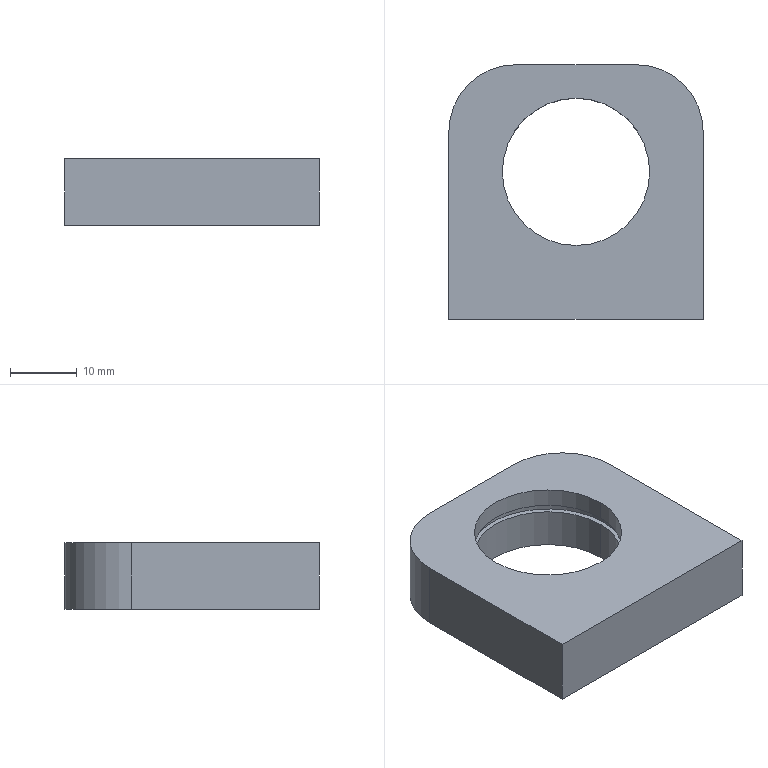Part | STEP file | 1 solid | 16 faces | box 38 x 38 x 10 mm | volume 10145 mm3 | cylinder 8 | plane 8 | commonest cylinder face diameters 22 x4 20 x2 23.5 x2
STEP:
#1=CARTESIAN_POINT('',(0.,0.,0.));
#2=DIRECTION('',(0.,0.,1.));
#3=DIRECTION('',(1.,0.,0.));
#4=AXIS2_PLACEMENT_3D('',#1,#2,#3);
#5=CARTESIAN_POINT('',(-11.75,3.,7.2));
#6=VERTEX_POINT('',#5);
#7=CARTESIAN_POINT('',(-11.75,3.,6.));
#8=VERTEX_POINT('',#7);
#9=CARTESIAN_POINT('',(-11.75,3.,7.2));
#10=DIRECTION('',(0.,0.,-1.));
#11=VECTOR('',#10,1.);
#12=LINE('',#9,#11);
#13=CARTESIAN_POINT('',(0.,3.,7.2));
#14=DIRECTION('',(0.,0.,-1.));
#15=DIRECTION('',(-1.,0.,0.));
#16=AXIS2_PLACEMENT_3D('',#13,#14,#15);
#17=CYLINDRICAL_SURFACE('',#16,11.75);
#18=CARTESIAN_POINT('',(6.283,0.));
#19=DIRECTION('',(0.,1.));
#20=VECTOR('',#19,1.);
#21=LINE('',#18,#20);
#22=(GEOMETRIC_REPRESENTATION_CONTEXT(2)PARAMETRIC_REPRESENTATION_CONTEXT()REPRESENTATION_CONTEXT('',''));
#23=DEFINITIONAL_REPRESENTATION('',(#21),#22);
#24=PCURVE('',#17,#23);
#25=CARTESIAN_POINT('',(0.,3.,7.2));
#26=DIRECTION('',(0.,0.,-1.));
#27=DIRECTION('',(-1.,0.,0.));
#28=AXIS2_PLACEMENT_3D('',#25,#26,#27);
#29=CYLINDRICAL_SURFACE('',#28,11.75);
#30=CARTESIAN_POINT('',(0.,0.));
#31=DIRECTION('',(0.,1.));
#32=VECTOR('',#31,1.);
#33=LINE('',#30,#32);
#34=(GEOMETRIC_REPRESENTATION_CONTEXT(2)PARAMETRIC_REPRESENTATION_CONTEXT()REPRESENTATION_CONTEXT('',''));
#35=DEFINITIONAL_REPRESENTATION('',(#33),#34);
#36=PCURVE('',#29,#35);
#37=SURFACE_CURVE('',#12,(#24,#36),.PCURVE_S1.);
#38=EDGE_CURVE('',#6,#8,#37,.T.);
#39=ORIENTED_EDGE('',*,*,#38,.T.);
#40=CARTESIAN_POINT('',(11.75,3.,6.));
#41=VERTEX_POINT('',#40);
#42=CARTESIAN_POINT('',(0.,3.,6.));
#43=DIRECTION('',(0.,0.,-1.));
#44=DIRECTION('',(-1.,0.,0.));
#45=AXIS2_PLACEMENT_3D('',#42,#43,#44);
#46=CIRCLE('',#45,11.75);
#47=CARTESIAN_POINT('',(0.,1.2));
#48=DIRECTION('',(1.,0.));
#49=VECTOR('',#48,1.);
#50=LINE('',#47,#49);
#51=(GEOMETRIC_REPRESENTATION_CONTEXT(2)PARAMETRIC_REPRESENTATION_CONTEXT()REPRESENTATION_CONTEXT('',''));
#52=DEFINITIONAL_REPRESENTATION('',(#50),#51);
#53=PCURVE('',#17,#52);
#54=CARTESIAN_POINT('',(0.,3.,6.));
#55=DIRECTION('',(0.,0.,-1.));
#56=DIRECTION('',(-1.,0.,0.));
#57=AXIS2_PLACEMENT_3D('',#54,#55,#56);
#58=PLANE('',#57);
#59=CARTESIAN_POINT('',(0.,0.));
#60=DIRECTION('',(1.,0.));
#61=AXIS2_PLACEMENT_2D('',#59,#60);
#62=CIRCLE('',#61,11.75);
#63=(GEOMETRIC_REPRESENTATION_CONTEXT(2)PARAMETRIC_REPRESENTATION_CONTEXT()REPRESENTATION_CONTEXT('',''));
#64=DEFINITIONAL_REPRESENTATION('',(#62),#63);
#65=PCURVE('',#58,#64);
#66=SURFACE_CURVE('',#46,(#53,#65),.PCURVE_S1.);
#67=EDGE_CURVE('',#41,#8,#66,.T.);
#68=ORIENTED_EDGE('',*,*,#67,.F.);
#69=CARTESIAN_POINT('',(11.75,3.,7.2));
#70=VERTEX_POINT('',#69);
#71=CARTESIAN_POINT('',(11.75,3.,7.2));
#72=DIRECTION('',(0.,0.,-1.));
#73=VECTOR('',#72,1.);
#74=LINE('',#71,#73);
#75=CARTESIAN_POINT('',(3.142,0.));
#76=DIRECTION('',(0.,1.));
#77=VECTOR('',#76,1.);
#78=LINE('',#75,#77);
#79=(GEOMETRIC_REPRESENTATION_CONTEXT(2)PARAMETRIC_REPRESENTATION_CONTEXT()REPRESENTATION_CONTEXT('',''));
#80=DEFINITIONAL_REPRESENTATION('',(#78),#79);
#81=PCURVE('',#17,#80);
#82=CARTESIAN_POINT('',(3.142,0.));
#83=DIRECTION('',(0.,1.));
#84=VECTOR('',#83,1.);
#85=LINE('',#82,#84);
#86=(GEOMETRIC_REPRESENTATION_CONTEXT(2)PARAMETRIC_REPRESENTATION_CONTEXT()REPRESENTATION_CONTEXT('',''));
#87=DEFINITIONAL_REPRESENTATION('',(#85),#86);
#88=PCURVE('',#29,#87);
#89=SURFACE_CURVE('',#74,(#81,#88),.PCURVE_S1.);
#90=EDGE_CURVE('',#70,#41,#89,.T.);
#91=ORIENTED_EDGE('',*,*,#90,.F.);
#92=CARTESIAN_POINT('',(0.,3.,7.2));
#93=DIRECTION('',(0.,0.,-1.));
#94=DIRECTION('',(-1.,0.,0.));
#95=AXIS2_PLACEMENT_3D('',#92,#93,#94);
#96=CIRCLE('',#95,11.75);
#97=CARTESIAN_POINT('',(0.,0.));
#98=DIRECTION('',(1.,0.));
#99=VECTOR('',#98,1.);
#100=LINE('',#97,#99);
#101=(GEOMETRIC_REPRESENTATION_CONTEXT(2)PARAMETRIC_REPRESENTATION_CONTEXT()REPRESENTATION_CONTEXT('',''));
#102=DEFINITIONAL_REPRESENTATION('',(#100),#101);
#103=PCURVE('',#17,#102);
#104=CARTESIAN_POINT('',(0.,3.,7.2));
#105=DIRECTION('',(0.,0.,-1.));
#106=DIRECTION('',(-1.,0.,0.));
#107=AXIS2_PLACEMENT_3D('',#104,#105,#106);
#108=PLANE('',#107);
#109=CARTESIAN_POINT('',(0.,0.));
#110=DIRECTION('',(1.,0.));
#111=AXIS2_PLACEMENT_2D('',#109,#110);
#112=CIRCLE('',#111,11.75);
#113=(GEOMETRIC_REPRESENTATION_CONTEXT(2)PARAMETRIC_REPRESENTATION_CONTEXT()REPRESENTATION_CONTEXT('',''));
#114=DEFINITIONAL_REPRESENTATION('',(#112),#113);
#115=PCURVE('',#108,#114);
#116=SURFACE_CURVE('',#96,(#103,#115),.PCURVE_S1.);
#117=EDGE_CURVE('',#70,#6,#116,.T.);
#118=ORIENTED_EDGE('',*,*,#117,.T.);
#119=EDGE_LOOP('',(#39,#68,#91,#118));
#120=FACE_BOUND('',#119,.F.);
#121=ADVANCED_FACE('',(#120),#17,.F.);
#122=CARTESIAN_POINT('',(-11.,3.,6.));
#123=VERTEX_POINT('',#122);
#124=CARTESIAN_POINT('',(-11.,3.,0.));
#125=VERTEX_POINT('',#124);
#126=CARTESIAN_POINT('',(-11.,3.,10.));
#127=DIRECTION('',(0.,0.,-1.));
#128=VECTOR('',#127,1.);
#129=LINE('',#126,#128);
#130=CARTESIAN_POINT('',(0.,3.,10.));
#131=DIRECTION('',(0.,0.,-1.));
#132=DIRECTION('',(-1.,0.,0.));
#133=AXIS2_PLACEMENT_3D('',#130,#131,#132);
#134=CYLINDRICAL_SURFACE('',#133,11.);
#135=CARTESIAN_POINT('',(6.283,0.));
#136=DIRECTION('',(0.,1.));
#137=VECTOR('',#136,1.);
#138=LINE('',#135,#137);
#139=(GEOMETRIC_REPRESENTATION_CONTEXT(2)PARAMETRIC_REPRESENTATION_CONTEXT()REPRESENTATION_CONTEXT('',''));
#140=DEFINITIONAL_REPRESENTATION('',(#138),#139);
#141=PCURVE('',#134,#140);
#142=CARTESIAN_POINT('',(0.,3.,10.));
#143=DIRECTION('',(0.,0.,-1.));
#144=DIRECTION('',(-1.,0.,0.));
#145=AXIS2_PLACEMENT_3D('',#142,#143,#144);
#146=CYLINDRICAL_SURFACE('',#145,11.);
#147=CARTESIAN_POINT('',(0.,0.));
#148=DIRECTION('',(0.,1.));
#149=VECTOR('',#148,1.);
#150=LINE('',#147,#149);
#151=(GEOMETRIC_REPRESENTATION_CONTEXT(2)PARAMETRIC_REPRESENTATION_CONTEXT()REPRESENTATION_CONTEXT('',''));
#152=DEFINITIONAL_REPRESENTATION('',(#150),#151);
#153=PCURVE('',#146,#152);
#154=SURFACE_CURVE('',#129,(#141,#153),.PCURVE_S1.);
#155=EDGE_CURVE('',#123,#125,#154,.T.);
#156=ORIENTED_EDGE('',*,*,#155,.T.);
#157=CARTESIAN_POINT('',(11.,3.,0.));
#158=VERTEX_POINT('',#157);
#159=CARTESIAN_POINT('',(0.,3.,0.));
#160=DIRECTION('',(0.,0.,-1.));
#161=DIRECTION('',(-1.,0.,0.));
#162=AXIS2_PLACEMENT_3D('',#159,#160,#161);
#163=CIRCLE('',#162,11.);
#164=CARTESIAN_POINT('',(0.,10.));
#165=DIRECTION('',(1.,0.));
#166=VECTOR('',#165,1.);
#167=LINE('',#164,#166);
#168=(GEOMETRIC_REPRESENTATION_CONTEXT(2)PARAMETRIC_REPRESENTATION_CONTEXT()REPRESENTATION_CONTEXT('',''));
#169=DEFINITIONAL_REPRESENTATION('',(#167),#168);
#170=PCURVE('',#134,#169);
#171=CARTESIAN_POINT('',(-9.,9.,0.));
#172=DIRECTION('',(0.,0.,1.));
#173=DIRECTION('',(1.,0.,0.));
#174=AXIS2_PLACEMENT_3D('',#171,#172,#173);
#175=PLANE('',#174);
#176=CARTESIAN_POINT('',(-2.,-6.));
#177=CARTESIAN_POINT('',(-2.,13.053));
#178=CARTESIAN_POINT('',(14.5,3.526));
#179=CARTESIAN_POINT('',(31.,-6.));
#180=CARTESIAN_POINT('',(14.5,-15.526));
#181=CARTESIAN_POINT('',(-2.,-25.053));
#182=CARTESIAN_POINT('',(-2.,-6.));
#183=(BOUNDED_CURVE()B_SPLINE_CURVE(2,(#176,#177,#178,#179,#180,#181,#182),.UNSPECIFIED.,.T.,.F.)B_SPLINE_CURVE_WITH_KNOTS((1,2,2,2,2,1),(-2.094,0.,2.094,4.189,6.283,8.378),.UNSPECIFIED.)CURVE()GEOMETRIC_REPRESENTATION_ITEM()RATIONAL_B_SPLINE_CURVE((1.,0.5,1.,0.5,1.,0.5,1.))REPRESENTATION_ITEM(''));
#184=(GEOMETRIC_REPRESENTATION_CONTEXT(2)PARAMETRIC_REPRESENTATION_CONTEXT()REPRESENTATION_CONTEXT('',''));
#185=DEFINITIONAL_REPRESENTATION('',(#183),#184);
#186=PCURVE('',#175,#185);
#187=SURFACE_CURVE('',#163,(#170,#186),.PCURVE_S1.);
#188=EDGE_CURVE('',#158,#125,#187,.T.);
#189=ORIENTED_EDGE('',*,*,#188,.F.);
#190=CARTESIAN_POINT('',(11.,3.,6.));
#191=VERTEX_POINT('',#190);
#192=CARTESIAN_POINT('',(11.,3.,10.));
#193=DIRECTION('',(0.,0.,-1.));
#194=VECTOR('',#193,1.);
#195=LINE('',#192,#194);
#196=CARTESIAN_POINT('',(3.142,0.));
#197=DIRECTION('',(0.,1.));
#198=VECTOR('',#197,1.);
#199=LINE('',#196,#198);
#200=(GEOMETRIC_REPRESENTATION_CONTEXT(2)PARAMETRIC_REPRESENTATION_CONTEXT()REPRESENTATION_CONTEXT('',''));
#201=DEFINITIONAL_REPRESENTATION('',(#199),#200);
#202=PCURVE('',#134,#201);
#203=CARTESIAN_POINT('',(3.142,0.));
#204=DIRECTION('',(0.,1.));
#205=VECTOR('',#204,1.);
#206=LINE('',#203,#205);
#207=(GEOMETRIC_REPRESENTATION_CONTEXT(2)PARAMETRIC_REPRESENTATION_CONTEXT()REPRESENTATION_CONTEXT('',''));
#208=DEFINITIONAL_REPRESENTATION('',(#206),#207);
#209=PCURVE('',#146,#208);
#210=SURFACE_CURVE('',#195,(#202,#209),.PCURVE_S1.);
#211=EDGE_CURVE('',#191,#158,#210,.T.);
#212=ORIENTED_EDGE('',*,*,#211,.F.);
#213=CARTESIAN_POINT('',(0.,3.,6.));
#214=DIRECTION('',(0.,0.,-1.));
#215=DIRECTION('',(-1.,0.,0.));
#216=AXIS2_PLACEMENT_3D('',#213,#214,#215);
#217=CIRCLE('',#216,11.);
#218=CARTESIAN_POINT('',(0.,4.));
#219=DIRECTION('',(1.,0.));
#220=VECTOR('',#219,1.);
#221=LINE('',#218,#220);
#222=(GEOMETRIC_REPRESENTATION_CONTEXT(2)PARAMETRIC_REPRESENTATION_CONTEXT()REPRESENTATION_CONTEXT('',''));
#223=DEFINITIONAL_REPRESENTATION('',(#221),#222);
#224=PCURVE('',#134,#223);
#225=CARTESIAN_POINT('',(0.,0.));
#226=DIRECTION('',(1.,0.));
#227=AXIS2_PLACEMENT_2D('',#225,#226);
#228=CIRCLE('',#227,11.);
#229=(GEOMETRIC_REPRESENTATION_CONTEXT(2)PARAMETRIC_REPRESENTATION_CONTEXT()REPRESENTATION_CONTEXT('',''));
#230=DEFINITIONAL_REPRESENTATION('',(#228),#229);
#231=PCURVE('',#58,#230);
#232=SURFACE_CURVE('',#217,(#224,#231),.PCURVE_S1.);
#233=EDGE_CURVE('',#191,#123,#232,.T.);
#234=ORIENTED_EDGE('',*,*,#233,.T.);
#235=EDGE_LOOP('',(#156,#189,#212,#234));
#236=FACE_BOUND('',#235,.F.);
#237=ADVANCED_FACE('',(#236),#134,.F.);
#238=CARTESIAN_POINT('',(-11.,3.,10.));
#239=VERTEX_POINT('',#238);
#240=CARTESIAN_POINT('',(-11.,3.,7.2));
#241=VERTEX_POINT('',#240);
#242=CARTESIAN_POINT('',(-11.,3.,10.));
#243=DIRECTION('',(0.,0.,-1.));
#244=VECTOR('',#243,1.);
#245=LINE('',#242,#244);
#246=CARTESIAN_POINT('',(0.,3.,10.));
#247=DIRECTION('',(0.,0.,-1.));
#248=DIRECTION('',(-1.,0.,0.));
#249=AXIS2_PLACEMENT_3D('',#246,#247,#248);
#250=CYLINDRICAL_SURFACE('',#249,11.);
#251=CARTESIAN_POINT('',(6.283,0.));
#252=DIRECTION('',(0.,1.));
#253=VECTOR('',#252,1.);
#254=LINE('',#251,#253);
#255=(GEOMETRIC_REPRESENTATION_CONTEXT(2)PARAMETRIC_REPRESENTATION_CONTEXT()REPRESENTATION_CONTEXT('',''));
#256=DEFINITIONAL_REPRESENTATION('',(#254),#255);
#257=PCURVE('',#250,#256);
#258=CARTESIAN_POINT('',(0.,3.,10.));
#259=DIRECTION('',(0.,0.,-1.));
#260=DIRECTION('',(-1.,0.,0.));
#261=AXIS2_PLACEMENT_3D('',#258,#259,#260);
#262=CYLINDRICAL_SURFACE('',#261,11.);
#263=CARTESIAN_POINT('',(0.,0.));
#264=DIRECTION('',(0.,1.));
#265=VECTOR('',#264,1.);
#266=LINE('',#263,#265);
#267=(GEOMETRIC_REPRESENTATION_CONTEXT(2)PARAMETRIC_REPRESENTATION_CONTEXT()REPRESENTATION_CONTEXT('',''));
#268=DEFINITIONAL_REPRESENTATION('',(#266),#267);
#269=PCURVE('',#262,#268);
#270=SURFACE_CURVE('',#245,(#257,#269),.PCURVE_S1.);
#271=EDGE_CURVE('',#239,#241,#270,.T.);
#272=ORIENTED_EDGE('',*,*,#271,.T.);
#273=CARTESIAN_POINT('',(11.,3.,7.2));
#274=VERTEX_POINT('',#273);
#275=CARTESIAN_POINT('',(0.,3.,7.2));
#276=DIRECTION('',(0.,0.,-1.));
#277=DIRECTION('',(-1.,0.,0.));
#278=AXIS2_PLACEMENT_3D('',#275,#276,#277);
#279=CIRCLE('',#278,11.);
#280=CARTESIAN_POINT('',(0.,2.8));
#281=DIRECTION('',(1.,0.));
#282=VECTOR('',#281,1.);
#283=LINE('',#280,#282);
#284=(GEOMETRIC_REPRESENTATION_CONTEXT(2)PARAMETRIC_REPRESENTATION_CONTEXT()REPRESENTATION_CONTEXT('',''));
#285=DEFINITIONAL_REPRESENTATION('',(#283),#284);
#286=PCURVE('',#250,#285);
#287=CARTESIAN_POINT('',(0.,0.));
#288=DIRECTION('',(1.,0.));
#289=AXIS2_PLACEMENT_2D('',#287,#288);
#290=CIRCLE('',#289,11.);
#291=(GEOMETRIC_REPRESENTATION_CONTEXT(2)PARAMETRIC_REPRESENTATION_CONTEXT()REPRESENTATION_CONTEXT('',''));
#292=DEFINITIONAL_REPRESENTATION('',(#290),#291);
#293=PCURVE('',#108,#292);
#294=SURFACE_CURVE('',#279,(#286,#293),.PCURVE_S1.);
#295=EDGE_CURVE('',#274,#241,#294,.T.);
#296=ORIENTED_EDGE('',*,*,#295,.F.);
#297=CARTESIAN_POINT('',(11.,3.,10.));
#298=VERTEX_POINT('',#297);
#299=CARTESIAN_POINT('',(11.,3.,10.));
#300=DIRECTION('',(0.,0.,-1.));
#301=VECTOR('',#300,1.);
#302=LINE('',#299,#301);
#303=CARTESIAN_POINT('',(3.142,0.));
#304=DIRECTION('',(0.,1.));
#305=VECTOR('',#304,1.);
#306=LINE('',#303,#305);
#307=(GEOMETRIC_REPRESENTATION_CONTEXT(2)PARAMETRIC_REPRESENTATION_CONTEXT()REPRESENTATION_CONTEXT('',''));
#308=DEFINITIONAL_REPRESENTATION('',(#306),#307);
#309=PCURVE('',#250,#308);
#310=CARTESIAN_POINT('',(3.142,0.));
#311=DIRECTION('',(0.,1.));
#312=VECTOR('',#311,1.);
#313=LINE('',#310,#312);
#314=(GEOMETRIC_REPRESENTATION_CONTEXT(2)PARAMETRIC_REPRESENTATION_CONTEXT()REPRESENTATION_CONTEXT('',''));
#315=DEFINITIONAL_REPRESENTATION('',(#313),#314);
#316=PCURVE('',#262,#315);
#317=SURFACE_CURVE('',#302,(#309,#316),.PCURVE_S1.);
#318=EDGE_CURVE('',#298,#274,#317,.T.);
#319=ORIENTED_EDGE('',*,*,#318,.F.);
#320=CARTESIAN_POINT('',(0.,3.,10.));
#321=DIRECTION('',(0.,0.,-1.));
#322=DIRECTION('',(-1.,0.,0.));
#323=AXIS2_PLACEMENT_3D('',#320,#321,#322);
#324=CIRCLE('',#323,11.);
#325=CARTESIAN_POINT('',(0.,0.));
#326=DIRECTION('',(1.,0.));
#327=VECTOR('',#326,1.);
#328=LINE('',#325,#327);
#329=(GEOMETRIC_REPRESENTATION_CONTEXT(2)PARAMETRIC_REPRESENTATION_CONTEXT()REPRESENTATION_CONTEXT('',''));
#330=DEFINITIONAL_REPRESENTATION('',(#328),#329);
#331=PCURVE('',#250,#330);
#332=CARTESIAN_POINT('',(-9.,9.,10.));
#333=DIRECTION('',(0.,0.,1.));
#334=DIRECTION('',(1.,0.,0.));
#335=AXIS2_PLACEMENT_3D('',#332,#333,#334);
#336=PLANE('',#335);
#337=CARTESIAN_POINT('',(-2.,-6.));
#338=CARTESIAN_POINT('',(-2.,13.053));
#339=CARTESIAN_POINT('',(14.5,3.526));
#340=CARTESIAN_POINT('',(31.,-6.));
#341=CARTESIAN_POINT('',(14.5,-15.526));
#342=CARTESIAN_POINT('',(-2.,-25.053));
#343=CARTESIAN_POINT('',(-2.,-6.));
#344=(BOUNDED_CURVE()B_SPLINE_CURVE(2,(#337,#338,#339,#340,#341,#342,#343),.UNSPECIFIED.,.T.,.F.)B_SPLINE_CURVE_WITH_KNOTS((1,2,2,2,2,1),(-2.094,0.,2.094,4.189,6.283,8.378),.UNSPECIFIED.)CURVE()GEOMETRIC_REPRESENTATION_ITEM()RATIONAL_B_SPLINE_CURVE((1.,0.5,1.,0.5,1.,0.5,1.))REPRESENTATION_ITEM(''));
#345=(GEOMETRIC_REPRESENTATION_CONTEXT(2)PARAMETRIC_REPRESENTATION_CONTEXT()REPRESENTATION_CONTEXT('',''));
#346=DEFINITIONAL_REPRESENTATION('',(#344),#345);
#347=PCURVE('',#336,#346);
#348=SURFACE_CURVE('',#324,(#331,#347),.PCURVE_S1.);
#349=EDGE_CURVE('',#298,#239,#348,.T.);
#350=ORIENTED_EDGE('',*,*,#349,.T.);
#351=EDGE_LOOP('',(#272,#296,#319,#350));
#352=FACE_BOUND('',#351,.F.);
#353=ADVANCED_FACE('',(#352),#250,.F.);
#354=CARTESIAN_POINT('',(0.,3.,7.2));
#355=DIRECTION('',(0.,0.,-1.));
#356=DIRECTION('',(-1.,0.,0.));
#357=AXIS2_PLACEMENT_3D('',#354,#355,#356);
#358=CIRCLE('',#357,11.);
#359=CARTESIAN_POINT('',(0.,2.8));
#360=DIRECTION('',(1.,0.));
#361=VECTOR('',#360,1.);
#362=LINE('',#359,#361);
#363=(GEOMETRIC_REPRESENTATION_CONTEXT(2)PARAMETRIC_REPRESENTATION_CONTEXT()REPRESENTATION_CONTEXT('',''));
#364=DEFINITIONAL_REPRESENTATION('',(#362),#363);
#365=PCURVE('',#262,#364);
#366=CARTESIAN_POINT('',(0.,0.));
#367=DIRECTION('',(1.,0.));
#368=AXIS2_PLACEMENT_2D('',#366,#367);
#369=CIRCLE('',#368,11.);
#370=(GEOMETRIC_REPRESENTATION_CONTEXT(2)PARAMETRIC_REPRESENTATION_CONTEXT()REPRESENTATION_CONTEXT('',''));
#371=DEFINITIONAL_REPRESENTATION('',(#369),#370);
#372=PCURVE('',#108,#371);
#373=SURFACE_CURVE('',#358,(#365,#372),.PCURVE_S1.);
#374=EDGE_CURVE('',#241,#274,#373,.T.);
#375=ORIENTED_EDGE('',*,*,#374,.F.);
#376=ORIENTED_EDGE('',*,*,#271,.F.);
#377=CARTESIAN_POINT('',(0.,3.,10.));
#378=DIRECTION('',(0.,0.,-1.));
#379=DIRECTION('',(-1.,0.,0.));
#380=AXIS2_PLACEMENT_3D('',#377,#378,#379);
#381=CIRCLE('',#380,11.);
#382=CARTESIAN_POINT('',(0.,0.));
#383=DIRECTION('',(1.,0.));
#384=VECTOR('',#383,1.);
#385=LINE('',#382,#384);
#386=(GEOMETRIC_REPRESENTATION_CONTEXT(2)PARAMETRIC_REPRESENTATION_CONTEXT()REPRESENTATION_CONTEXT('',''));
#387=DEFINITIONAL_REPRESENTATION('',(#385),#386);
#388=PCURVE('',#262,#387);
#389=CARTESIAN_POINT('',(-2.,-6.));
#390=CARTESIAN_POINT('',(-2.,13.053));
#391=CARTESIAN_POINT('',(14.5,3.526));
#392=CARTESIAN_POINT('',(31.,-6.));
#393=CARTESIAN_POINT('',(14.5,-15.526));
#394=CARTESIAN_POINT('',(-2.,-25.053));
#395=CARTESIAN_POINT('',(-2.,-6.));
#396=(BOUNDED_CURVE()B_SPLINE_CURVE(2,(#389,#390,#391,#392,#393,#394,#395),.UNSPECIFIED.,.T.,.F.)B_SPLINE_CURVE_WITH_KNOTS((1,2,2,2,2,1),(-2.094,0.,2.094,4.189,6.283,8.378),.UNSPECIFIED.)CURVE()GEOMETRIC_REPRESENTATION_ITEM()RATIONAL_B_SPLINE_CURVE((1.,0.5,1.,0.5,1.,0.5,1.))REPRESENTATION_ITEM(''));
#397=(GEOMETRIC_REPRESENTATION_CONTEXT(2)PARAMETRIC_REPRESENTATION_CONTEXT()REPRESENTATION_CONTEXT('',''));
#398=DEFINITIONAL_REPRESENTATION('',(#396),#397);
#399=PCURVE('',#336,#398);
#400=SURFACE_CURVE('',#381,(#388,#399),.PCURVE_S1.);
#401=EDGE_CURVE('',#239,#298,#400,.T.);
#402=ORIENTED_EDGE('',*,*,#401,.T.);
#403=ORIENTED_EDGE('',*,*,#318,.T.);
#404=EDGE_LOOP('',(#375,#376,#402,#403));
#405=FACE_BOUND('',#404,.F.);
#406=ADVANCED_FACE('',(#405),#262,.F.);
#407=CARTESIAN_POINT('',(19.,-19.,0.));
#408=VERTEX_POINT('',#407);
#409=CARTESIAN_POINT('',(19.,9.,0.));
#410=VERTEX_POINT('',#409);
#411=CARTESIAN_POINT('',(19.,9.,0.));
#412=DIRECTION('',(0.,1.,0.));
#413=VECTOR('',#412,1.);
#414=LINE('',#411,#413);
#415=CARTESIAN_POINT('',(19.,9.,10.));
#416=DIRECTION('',(-1.,0.,0.));
#417=DIRECTION('',(0.,-1.,0.));
#418=AXIS2_PLACEMENT_3D('',#415,#416,#417);
#419=PLANE('',#418);
#420=CARTESIAN_POINT('',(0.,-10.));
#421=DIRECTION('',(-1.,0.));
#422=VECTOR('',#421,1.);
#423=LINE('',#420,#422);
#424=(GEOMETRIC_REPRESENTATION_CONTEXT(2)PARAMETRIC_REPRESENTATION_CONTEXT()REPRESENTATION_CONTEXT('',''));
#425=DEFINITIONAL_REPRESENTATION('',(#423),#424);
#426=PCURVE('',#419,#425);
#427=CARTESIAN_POINT('',(28.,0.));
#428=DIRECTION('',(0.,1.));
#429=VECTOR('',#428,1.);
#430=LINE('',#427,#429);
#431=(GEOMETRIC_REPRESENTATION_CONTEXT(2)PARAMETRIC_REPRESENTATION_CONTEXT()REPRESENTATION_CONTEXT('',''));
#432=DEFINITIONAL_REPRESENTATION('',(#430),#431);
#433=PCURVE('',#175,#432);
#434=SURFACE_CURVE('',#414,(#426,#433),.PCURVE_S1.);
#435=EDGE_CURVE('',#408,#410,#434,.T.);
#436=ORIENTED_EDGE('',*,*,#435,.T.);
#437=CARTESIAN_POINT('',(19.,9.,10.));
#438=VERTEX_POINT('',#437);
#439=CARTESIAN_POINT('',(19.,9.,10.));
#440=DIRECTION('',(0.,0.,-1.));
#441=VECTOR('',#440,1.);
#442=LINE('',#439,#441);
#443=CARTESIAN_POINT('',(0.,0.));
#444=DIRECTION('',(0.,-1.));
#445=VECTOR('',#444,1.);
#446=LINE('',#443,#445);
#447=(GEOMETRIC_REPRESENTATION_CONTEXT(2)PARAMETRIC_REPRESENTATION_CONTEXT()REPRESENTATION_CONTEXT('',''));
#448=DEFINITIONAL_REPRESENTATION('',(#446),#447);
#449=PCURVE('',#419,#448);
#450=CARTESIAN_POINT('',(9.,9.,10.));
#451=DIRECTION('',(0.,0.,-1.));
#452=DIRECTION('',(-1.,0.,0.));
#453=AXIS2_PLACEMENT_3D('',#450,#451,#452);
#454=CYLINDRICAL_SURFACE('',#453,10.);
#455=CARTESIAN_POINT('',(3.142,0.));
#456=DIRECTION('',(0.,1.));
#457=VECTOR('',#456,1.);
#458=LINE('',#455,#457);
#459=(GEOMETRIC_REPRESENTATION_CONTEXT(2)PARAMETRIC_REPRESENTATION_CONTEXT()REPRESENTATION_CONTEXT('',''));
#460=DEFINITIONAL_REPRESENTATION('',(#458),#459);
#461=PCURVE('',#454,#460);
#462=SURFACE_CURVE('',#442,(#449,#461),.PCURVE_S1.);
#463=EDGE_CURVE('',#438,#410,#462,.T.);
#464=ORIENTED_EDGE('',*,*,#463,.F.);
#465=CARTESIAN_POINT('',(19.,-19.,10.));
#466=VERTEX_POINT('',#465);
#467=CARTESIAN_POINT('',(19.,9.,10.));
#468=DIRECTION('',(0.,1.,0.));
#469=VECTOR('',#468,1.);
#470=LINE('',#467,#469);
#471=CARTESIAN_POINT('',(0.,0.));
#472=DIRECTION('',(-1.,0.));
#473=VECTOR('',#472,1.);
#474=LINE('',#471,#473);
#475=(GEOMETRIC_REPRESENTATION_CONTEXT(2)PARAMETRIC_REPRESENTATION_CONTEXT()REPRESENTATION_CONTEXT('',''));
#476=DEFINITIONAL_REPRESENTATION('',(#474),#475);
#477=PCURVE('',#419,#476);
#478=CARTESIAN_POINT('',(28.,0.));
#479=DIRECTION('',(0.,1.));
#480=VECTOR('',#479,1.);
#481=LINE('',#478,#480);
#482=(GEOMETRIC_REPRESENTATION_CONTEXT(2)PARAMETRIC_REPRESENTATION_CONTEXT()REPRESENTATION_CONTEXT('',''));
#483=DEFINITIONAL_REPRESENTATION('',(#481),#482);
#484=PCURVE('',#336,#483);
#485=SURFACE_CURVE('',#470,(#477,#484),.PCURVE_S1.);
#486=EDGE_CURVE('',#466,#438,#485,.T.);
#487=ORIENTED_EDGE('',*,*,#486,.F.);
#488=CARTESIAN_POINT('',(19.,-19.,10.));
#489=DIRECTION('',(0.,0.,-1.));
#490=VECTOR('',#489,1.);
#491=LINE('',#488,#490);
#492=CARTESIAN_POINT('',(28.,0.));
#493=DIRECTION('',(0.,-1.));
#494=VECTOR('',#493,1.);
#495=LINE('',#492,#494);
#496=(GEOMETRIC_REPRESENTATION_CONTEXT(2)PARAMETRIC_REPRESENTATION_CONTEXT()REPRESENTATION_CONTEXT('',''));
#497=DEFINITIONAL_REPRESENTATION('',(#495),#496);
#498=PCURVE('',#419,#497);
#499=CARTESIAN_POINT('',(-19.,-19.,10.));
#500=DIRECTION('',(0.,1.,0.));
#501=DIRECTION('',(0.,0.,1.));
#502=AXIS2_PLACEMENT_3D('',#499,#500,#501);
#503=PLANE('',#502);
#504=CARTESIAN_POINT('',(0.,38.));
#505=DIRECTION('',(-1.,0.));
#506=VECTOR('',#505,1.);
#507=LINE('',#504,#506);
#508=(GEOMETRIC_REPRESENTATION_CONTEXT(2)PARAMETRIC_REPRESENTATION_CONTEXT()REPRESENTATION_CONTEXT('',''));
#509=DEFINITIONAL_REPRESENTATION('',(#507),#508);
#510=PCURVE('',#503,#509);
#511=SURFACE_CURVE('',#491,(#498,#510),.PCURVE_S1.);
#512=EDGE_CURVE('',#466,#408,#511,.T.);
#513=ORIENTED_EDGE('',*,*,#512,.T.);
#514=EDGE_LOOP('',(#436,#464,#487,#513));
#515=FACE_BOUND('',#514,.T.);
#516=ADVANCED_FACE('',(#515),#419,.F.);
#517=CARTESIAN_POINT('',(9.,19.,0.));
#518=VERTEX_POINT('',#517);
#519=CARTESIAN_POINT('',(9.,9.,0.));
#520=DIRECTION('',(0.,0.,1.));
#521=DIRECTION('',(-1.,0.,0.));
#522=AXIS2_PLACEMENT_3D('',#519,#520,#521);
#523=CIRCLE('',#522,10.);
#524=CARTESIAN_POINT('',(6.283,10.));
#525=DIRECTION('',(-1.,0.));
#526=VECTOR('',#525,1.);
#527=LINE('',#524,#526);
#528=(GEOMETRIC_REPRESENTATION_CONTEXT(2)PARAMETRIC_REPRESENTATION_CONTEXT()REPRESENTATION_CONTEXT('',''));
#529=DEFINITIONAL_REPRESENTATION('',(#527),#528);
#530=PCURVE('',#454,#529);
#531=CARTESIAN_POINT('',(18.,0.));
#532=DIRECTION('',(-1.,0.));
#533=AXIS2_PLACEMENT_2D('',#531,#532);
#534=CIRCLE('',#533,10.);
#535=(GEOMETRIC_REPRESENTATION_CONTEXT(2)PARAMETRIC_REPRESENTATION_CONTEXT()REPRESENTATION_CONTEXT('',''));
#536=DEFINITIONAL_REPRESENTATION('',(#534),#535);
#537=PCURVE('',#175,#536);
#538=SURFACE_CURVE('',#523,(#530,#537),.PCURVE_S1.);
#539=EDGE_CURVE('',#410,#518,#538,.T.);
#540=ORIENTED_EDGE('',*,*,#539,.T.);
#541=CARTESIAN_POINT('',(9.,19.,10.));
#542=VERTEX_POINT('',#541);
#543=CARTESIAN_POINT('',(9.,19.,10.));
#544=DIRECTION('',(0.,0.,-1.));
#545=VECTOR('',#544,1.);
#546=LINE('',#543,#545);
#547=CARTESIAN_POINT('',(1.571,0.));
#548=DIRECTION('',(0.,1.));
#549=VECTOR('',#548,1.);
#550=LINE('',#547,#549);
#551=(GEOMETRIC_REPRESENTATION_CONTEXT(2)PARAMETRIC_REPRESENTATION_CONTEXT()REPRESENTATION_CONTEXT('',''));
#552=DEFINITIONAL_REPRESENTATION('',(#550),#551);
#553=PCURVE('',#454,#552);
#554=CARTESIAN_POINT('',(-9.,19.,10.));
#555=DIRECTION('',(0.,-1.,0.));
#556=DIRECTION('',(1.,0.,0.));
#557=AXIS2_PLACEMENT_3D('',#554,#555,#556);
#558=PLANE('',#557);
#559=CARTESIAN_POINT('',(18.,0.));
#560=DIRECTION('',(0.,-1.));
#561=VECTOR('',#560,1.);
#562=LINE('',#559,#561);
#563=(GEOMETRIC_REPRESENTATION_CONTEXT(2)PARAMETRIC_REPRESENTATION_CONTEXT()REPRESENTATION_CONTEXT('',''));
#564=DEFINITIONAL_REPRESENTATION('',(#562),#563);
#565=PCURVE('',#558,#564);
#566=SURFACE_CURVE('',#546,(#553,#565),.PCURVE_S1.);
#567=EDGE_CURVE('',#542,#518,#566,.T.);
#568=ORIENTED_EDGE('',*,*,#567,.F.);
#569=CARTESIAN_POINT('',(9.,9.,10.));
#570=DIRECTION('',(0.,0.,1.));
#571=DIRECTION('',(-1.,0.,0.));
#572=AXIS2_PLACEMENT_3D('',#569,#570,#571);
#573=CIRCLE('',#572,10.);
#574=CARTESIAN_POINT('',(6.283,0.));
#575=DIRECTION('',(-1.,0.));
#576=VECTOR('',#575,1.);
#577=LINE('',#574,#576);
#578=(GEOMETRIC_REPRESENTATION_CONTEXT(2)PARAMETRIC_REPRESENTATION_CONTEXT()REPRESENTATION_CONTEXT('',''));
#579=DEFINITIONAL_REPRESENTATION('',(#577),#578);
#580=PCURVE('',#454,#579);
#581=CARTESIAN_POINT('',(18.,0.));
#582=DIRECTION('',(-1.,0.));
#583=AXIS2_PLACEMENT_2D('',#581,#582);
#584=CIRCLE('',#583,10.);
#585=(GEOMETRIC_REPRESENTATION_CONTEXT(2)PARAMETRIC_REPRESENTATION_CONTEXT()REPRESENTATION_CONTEXT('',''));
#586=DEFINITIONAL_REPRESENTATION('',(#584),#585);
#587=PCURVE('',#336,#586);
#588=SURFACE_CURVE('',#573,(#580,#587),.PCURVE_S1.);
#589=EDGE_CURVE('',#438,#542,#588,.T.);
#590=ORIENTED_EDGE('',*,*,#589,.F.);
#591=ORIENTED_EDGE('',*,*,#463,.T.);
#592=EDGE_LOOP('',(#540,#568,#590,#591));
#593=FACE_BOUND('',#592,.T.);
#594=ADVANCED_FACE('',(#593),#454,.T.);
#595=CARTESIAN_POINT('',(-9.,19.,0.));
#596=VERTEX_POINT('',#595);
#597=CARTESIAN_POINT('',(-9.,19.,0.));
#598=DIRECTION('',(-1.,0.,0.));
#599=VECTOR('',#598,1.);
#600=LINE('',#597,#599);
#601=CARTESIAN_POINT('',(0.,-10.));
#602=DIRECTION('',(-1.,0.));
#603=VECTOR('',#602,1.);
#604=LINE('',#601,#603);
#605=(GEOMETRIC_REPRESENTATION_CONTEXT(2)PARAMETRIC_REPRESENTATION_CONTEXT()REPRESENTATION_CONTEXT('',''));
#606=DEFINITIONAL_REPRESENTATION('',(#604),#605);
#607=PCURVE('',#558,#606);
#608=CARTESIAN_POINT('',(0.,10.));
#609=DIRECTION('',(-1.,0.));
#610=VECTOR('',#609,1.);
#611=LINE('',#608,#610);
#612=(GEOMETRIC_REPRESENTATION_CONTEXT(2)PARAMETRIC_REPRESENTATION_CONTEXT()REPRESENTATION_CONTEXT('',''));
#613=DEFINITIONAL_REPRESENTATION('',(#611),#612);
#614=PCURVE('',#175,#613);
#615=SURFACE_CURVE('',#600,(#607,#614),.PCURVE_S1.);
#616=EDGE_CURVE('',#518,#596,#615,.T.);
#617=ORIENTED_EDGE('',*,*,#616,.T.);
#618=CARTESIAN_POINT('',(-9.,19.,10.));
#619=VERTEX_POINT('',#618);
#620=CARTESIAN_POINT('',(-9.,19.,10.));
#621=DIRECTION('',(0.,0.,-1.));
#622=VECTOR('',#621,1.);
#623=LINE('',#620,#622);
#624=CARTESIAN_POINT('',(0.,0.));
#625=DIRECTION('',(0.,-1.));
#626=VECTOR('',#625,1.);
#627=LINE('',#624,#626);
#628=(GEOMETRIC_REPRESENTATION_CONTEXT(2)PARAMETRIC_REPRESENTATION_CONTEXT()REPRESENTATION_CONTEXT('',''));
#629=DEFINITIONAL_REPRESENTATION('',(#627),#628);
#630=PCURVE('',#558,#629);
#631=CARTESIAN_POINT('',(-9.,9.,10.));
#632=DIRECTION('',(0.,0.,-1.));
#633=DIRECTION('',(-1.,0.,0.));
#634=AXIS2_PLACEMENT_3D('',#631,#632,#633);
#635=CYLINDRICAL_SURFACE('',#634,10.);
#636=CARTESIAN_POINT('',(1.571,0.));
#637=DIRECTION('',(0.,1.));
#638=VECTOR('',#637,1.);
#639=LINE('',#636,#638);
#640=(GEOMETRIC_REPRESENTATION_CONTEXT(2)PARAMETRIC_REPRESENTATION_CONTEXT()REPRESENTATION_CONTEXT('',''));
#641=DEFINITIONAL_REPRESENTATION('',(#639),#640);
#642=PCURVE('',#635,#641);
#643=SURFACE_CURVE('',#623,(#630,#642),.PCURVE_S1.);
#644=EDGE_CURVE('',#619,#596,#643,.T.);
#645=ORIENTED_EDGE('',*,*,#644,.F.);
#646=CARTESIAN_POINT('',(-9.,19.,10.));
#647=DIRECTION('',(-1.,0.,0.));
#648=VECTOR('',#647,1.);
#649=LINE('',#646,#648);
#650=CARTESIAN_POINT('',(0.,0.));
#651=DIRECTION('',(-1.,0.));
#652=VECTOR('',#651,1.);
#653=LINE('',#650,#652);
#654=(GEOMETRIC_REPRESENTATION_CONTEXT(2)PARAMETRIC_REPRESENTATION_CONTEXT()REPRESENTATION_CONTEXT('',''));
#655=DEFINITIONAL_REPRESENTATION('',(#653),#654);
#656=PCURVE('',#558,#655);
#657=CARTESIAN_POINT('',(0.,10.));
#658=DIRECTION('',(-1.,0.));
#659=VECTOR('',#658,1.);
#660=LINE('',#657,#659);
#661=(GEOMETRIC_REPRESENTATION_CONTEXT(2)PARAMETRIC_REPRESENTATION_CONTEXT()REPRESENTATION_CONTEXT('',''));
#662=DEFINITIONAL_REPRESENTATION('',(#660),#661);
#663=PCURVE('',#336,#662);
#664=SURFACE_CURVE('',#649,(#656,#663),.PCURVE_S1.);
#665=EDGE_CURVE('',#542,#619,#664,.T.);
#666=ORIENTED_EDGE('',*,*,#665,.F.);
#667=ORIENTED_EDGE('',*,*,#567,.T.);
#668=EDGE_LOOP('',(#617,#645,#666,#667));
#669=FACE_BOUND('',#668,.T.);
#670=ADVANCED_FACE('',(#669),#558,.F.);
#671=CARTESIAN_POINT('',(-19.,9.,0.));
#672=VERTEX_POINT('',#671);
#673=CARTESIAN_POINT('',(-9.,9.,0.));
#674=DIRECTION('',(0.,0.,1.));
#675=DIRECTION('',(1.,0.,0.));
#676=AXIS2_PLACEMENT_3D('',#673,#674,#675);
#677=CIRCLE('',#676,10.);
#678=CARTESIAN_POINT('',(3.142,10.));
#679=DIRECTION('',(-1.,0.));
#680=VECTOR('',#679,1.);
#681=LINE('',#678,#680);
#682=(GEOMETRIC_REPRESENTATION_CONTEXT(2)PARAMETRIC_REPRESENTATION_CONTEXT()REPRESENTATION_CONTEXT('',''));
#683=DEFINITIONAL_REPRESENTATION('',(#681),#682);
#684=PCURVE('',#635,#683);
#685=CARTESIAN_POINT('',(0.,0.));
#686=DIRECTION('',(1.,0.));
#687=AXIS2_PLACEMENT_2D('',#685,#686);
#688=CIRCLE('',#687,10.);
#689=(GEOMETRIC_REPRESENTATION_CONTEXT(2)PARAMETRIC_REPRESENTATION_CONTEXT()REPRESENTATION_CONTEXT('',''));
#690=DEFINITIONAL_REPRESENTATION('',(#688),#689);
#691=PCURVE('',#175,#690);
#692=SURFACE_CURVE('',#677,(#684,#691),.PCURVE_S1.);
#693=EDGE_CURVE('',#596,#672,#692,.T.);
#694=ORIENTED_EDGE('',*,*,#693,.T.);
#695=CARTESIAN_POINT('',(-19.,9.,10.));
#696=VERTEX_POINT('',#695);
#697=CARTESIAN_POINT('',(-19.,9.,10.));
#698=DIRECTION('',(0.,0.,-1.));
#699=VECTOR('',#698,1.);
#700=LINE('',#697,#699);
#701=CARTESIAN_POINT('',(0.,0.));
#702=DIRECTION('',(0.,1.));
#703=VECTOR('',#702,1.);
#704=LINE('',#701,#703);
#705=(GEOMETRIC_REPRESENTATION_CONTEXT(2)PARAMETRIC_REPRESENTATION_CONTEXT()REPRESENTATION_CONTEXT('',''));
#706=DEFINITIONAL_REPRESENTATION('',(#704),#705);
#707=PCURVE('',#635,#706);
#708=CARTESIAN_POINT('',(-19.,9.,10.));
#709=DIRECTION('',(1.,0.,0.));
#710=DIRECTION('',(0.,1.,0.));
#711=AXIS2_PLACEMENT_3D('',#708,#709,#710);
#712=PLANE('',#711);
#713=CARTESIAN_POINT('',(0.,0.));
#714=DIRECTION('',(0.,-1.));
#715=VECTOR('',#714,1.);
#716=LINE('',#713,#715);
#717=(GEOMETRIC_REPRESENTATION_CONTEXT(2)PARAMETRIC_REPRESENTATION_CONTEXT()REPRESENTATION_CONTEXT('',''));
#718=DEFINITIONAL_REPRESENTATION('',(#716),#717);
#719=PCURVE('',#712,#718);
#720=SURFACE_CURVE('',#700,(#707,#719),.PCURVE_S1.);
#721=EDGE_CURVE('',#696,#672,#720,.T.);
#722=ORIENTED_EDGE('',*,*,#721,.F.);
#723=CARTESIAN_POINT('',(-9.,9.,10.));
#724=DIRECTION('',(0.,0.,1.));
#725=DIRECTION('',(1.,0.,0.));
#726=AXIS2_PLACEMENT_3D('',#723,#724,#725);
#727=CIRCLE('',#726,10.);
#728=CARTESIAN_POINT('',(3.142,0.));
#729=DIRECTION('',(-1.,0.));
#730=VECTOR('',#729,1.);
#731=LINE('',#728,#730);
#732=(GEOMETRIC_REPRESENTATION_CONTEXT(2)PARAMETRIC_REPRESENTATION_CONTEXT()REPRESENTATION_CONTEXT('',''));
#733=DEFINITIONAL_REPRESENTATION('',(#731),#732);
#734=PCURVE('',#635,#733);
#735=CARTESIAN_POINT('',(0.,0.));
#736=DIRECTION('',(1.,0.));
#737=AXIS2_PLACEMENT_2D('',#735,#736);
#738=CIRCLE('',#737,10.);
#739=(GEOMETRIC_REPRESENTATION_CONTEXT(2)PARAMETRIC_REPRESENTATION_CONTEXT()REPRESENTATION_CONTEXT('',''));
#740=DEFINITIONAL_REPRESENTATION('',(#738),#739);
#741=PCURVE('',#336,#740);
#742=SURFACE_CURVE('',#727,(#734,#741),.PCURVE_S1.);
#743=EDGE_CURVE('',#619,#696,#742,.T.);
#744=ORIENTED_EDGE('',*,*,#743,.F.);
#745=ORIENTED_EDGE('',*,*,#644,.T.);
#746=EDGE_LOOP('',(#694,#722,#744,#745));
#747=FACE_BOUND('',#746,.T.);
#748=ADVANCED_FACE('',(#747),#635,.T.);
#749=CARTESIAN_POINT('',(-19.,-19.,0.));
#750=VERTEX_POINT('',#749);
#751=CARTESIAN_POINT('',(-19.,9.,0.));
#752=DIRECTION('',(0.,-1.,0.));
#753=VECTOR('',#752,1.);
#754=LINE('',#751,#753);
#755=CARTESIAN_POINT('',(0.,-10.));
#756=DIRECTION('',(-1.,0.));
#757=VECTOR('',#756,1.);
#758=LINE('',#755,#757);
#759=(GEOMETRIC_REPRESENTATION_CONTEXT(2)PARAMETRIC_REPRESENTATION_CONTEXT()REPRESENTATION_CONTEXT('',''));
#760=DEFINITIONAL_REPRESENTATION('',(#758),#759);
#761=PCURVE('',#712,#760);
#762=CARTESIAN_POINT('',(-10.,0.));
#763=DIRECTION('',(0.,-1.));
#764=VECTOR('',#763,1.);
#765=LINE('',#762,#764);
#766=(GEOMETRIC_REPRESENTATION_CONTEXT(2)PARAMETRIC_REPRESENTATION_CONTEXT()REPRESENTATION_CONTEXT('',''));
#767=DEFINITIONAL_REPRESENTATION('',(#765),#766);
#768=PCURVE('',#175,#767);
#769=SURFACE_CURVE('',#754,(#761,#768),.PCURVE_S1.);
#770=EDGE_CURVE('',#672,#750,#769,.T.);
#771=ORIENTED_EDGE('',*,*,#770,.T.);
#772=CARTESIAN_POINT('',(-19.,-19.,10.));
#773=VERTEX_POINT('',#772);
#774=CARTESIAN_POINT('',(-19.,-19.,10.));
#775=DIRECTION('',(0.,0.,-1.));
#776=VECTOR('',#775,1.);
#777=LINE('',#774,#776);
#778=CARTESIAN_POINT('',(-28.,0.));
#779=DIRECTION('',(0.,-1.));
#780=VECTOR('',#779,1.);
#781=LINE('',#778,#780);
#782=(GEOMETRIC_REPRESENTATION_CONTEXT(2)PARAMETRIC_REPRESENTATION_CONTEXT()REPRESENTATION_CONTEXT('',''));
#783=DEFINITIONAL_REPRESENTATION('',(#781),#782);
#784=PCURVE('',#712,#783);
#785=CARTESIAN_POINT('',(0.,0.));
#786=DIRECTION('',(-1.,0.));
#787=VECTOR('',#786,1.);
#788=LINE('',#785,#787);
#789=(GEOMETRIC_REPRESENTATION_CONTEXT(2)PARAMETRIC_REPRESENTATION_CONTEXT()REPRESENTATION_CONTEXT('',''));
#790=DEFINITIONAL_REPRESENTATION('',(#788),#789);
#791=PCURVE('',#503,#790);
#792=SURFACE_CURVE('',#777,(#784,#791),.PCURVE_S1.);
#793=EDGE_CURVE('',#773,#750,#792,.T.);
#794=ORIENTED_EDGE('',*,*,#793,.F.);
#795=CARTESIAN_POINT('',(-19.,9.,10.));
#796=DIRECTION('',(0.,-1.,0.));
#797=VECTOR('',#796,1.);
#798=LINE('',#795,#797);
#799=CARTESIAN_POINT('',(0.,0.));
#800=DIRECTION('',(-1.,0.));
#801=VECTOR('',#800,1.);
#802=LINE('',#799,#801);
#803=(GEOMETRIC_REPRESENTATION_CONTEXT(2)PARAMETRIC_REPRESENTATION_CONTEXT()REPRESENTATION_CONTEXT('',''));
#804=DEFINITIONAL_REPRESENTATION('',(#802),#803);
#805=PCURVE('',#712,#804);
#806=CARTESIAN_POINT('',(-10.,0.));
#807=DIRECTION('',(0.,-1.));
#808=VECTOR('',#807,1.);
#809=LINE('',#806,#808);
#810=(GEOMETRIC_REPRESENTATION_CONTEXT(2)PARAMETRIC_REPRESENTATION_CONTEXT()REPRESENTATION_CONTEXT('',''));
#811=DEFINITIONAL_REPRESENTATION('',(#809),#810);
#812=PCURVE('',#336,#811);
#813=SURFACE_CURVE('',#798,(#805,#812),.PCURVE_S1.);
#814=EDGE_CURVE('',#696,#773,#813,.T.);
#815=ORIENTED_EDGE('',*,*,#814,.F.);
#816=ORIENTED_EDGE('',*,*,#721,.T.);
#817=EDGE_LOOP('',(#771,#794,#815,#816));
#818=FACE_BOUND('',#817,.T.);
#819=ADVANCED_FACE('',(#818),#712,.F.);
#820=CARTESIAN_POINT('',(-19.,-19.,0.));
#821=DIRECTION('',(1.,0.,0.));
#822=VECTOR('',#821,1.);
#823=LINE('',#820,#822);
#824=CARTESIAN_POINT('',(-10.,0.));
#825=DIRECTION('',(0.,1.));
#826=VECTOR('',#825,1.);
#827=LINE('',#824,#826);
#828=(GEOMETRIC_REPRESENTATION_CONTEXT(2)PARAMETRIC_REPRESENTATION_CONTEXT()REPRESENTATION_CONTEXT('',''));
#829=DEFINITIONAL_REPRESENTATION('',(#827),#828);
#830=PCURVE('',#503,#829);
#831=CARTESIAN_POINT('',(-10.,-28.));
#832=DIRECTION('',(1.,0.));
#833=VECTOR('',#832,1.);
#834=LINE('',#831,#833);
#835=(GEOMETRIC_REPRESENTATION_CONTEXT(2)PARAMETRIC_REPRESENTATION_CONTEXT()REPRESENTATION_CONTEXT('',''));
#836=DEFINITIONAL_REPRESENTATION('',(#834),#835);
#837=PCURVE('',#175,#836);
#838=SURFACE_CURVE('',#823,(#830,#837),.PCURVE_S1.);
#839=EDGE_CURVE('',#750,#408,#838,.T.);
#840=ORIENTED_EDGE('',*,*,#839,.T.);
#841=ORIENTED_EDGE('',*,*,#512,.F.);
#842=CARTESIAN_POINT('',(-19.,-19.,10.));
#843=DIRECTION('',(1.,0.,0.));
#844=VECTOR('',#843,1.);
#845=LINE('',#842,#844);
#846=CARTESIAN_POINT('',(0.,0.));
#847=DIRECTION('',(0.,1.));
#848=VECTOR('',#847,1.);
#849=LINE('',#846,#848);
#850=(GEOMETRIC_REPRESENTATION_CONTEXT(2)PARAMETRIC_REPRESENTATION_CONTEXT()REPRESENTATION_CONTEXT('',''));
#851=DEFINITIONAL_REPRESENTATION('',(#849),#850);
#852=PCURVE('',#503,#851);
#853=CARTESIAN_POINT('',(-10.,-28.));
#854=DIRECTION('',(1.,0.));
#855=VECTOR('',#854,1.);
#856=LINE('',#853,#855);
#857=(GEOMETRIC_REPRESENTATION_CONTEXT(2)PARAMETRIC_REPRESENTATION_CONTEXT()REPRESENTATION_CONTEXT('',''));
#858=DEFINITIONAL_REPRESENTATION('',(#856),#857);
#859=PCURVE('',#336,#858);
#860=SURFACE_CURVE('',#845,(#852,#859),.PCURVE_S1.);
#861=EDGE_CURVE('',#773,#466,#860,.T.);
#862=ORIENTED_EDGE('',*,*,#861,.F.);
#863=ORIENTED_EDGE('',*,*,#793,.T.);
#864=EDGE_LOOP('',(#840,#841,#862,#863));
#865=FACE_BOUND('',#864,.T.);
#866=ADVANCED_FACE('',(#865),#503,.F.);
#867=ORIENTED_EDGE('',*,*,#401,.T.);
#868=ORIENTED_EDGE('',*,*,#349,.T.);
#869=EDGE_LOOP('',(#867,#868));
#870=FACE_BOUND('',#869,.T.);
#871=ORIENTED_EDGE('',*,*,#486,.T.);
#872=ORIENTED_EDGE('',*,*,#589,.T.);
#873=ORIENTED_EDGE('',*,*,#665,.T.);
#874=ORIENTED_EDGE('',*,*,#743,.T.);
#875=ORIENTED_EDGE('',*,*,#814,.T.);
#876=ORIENTED_EDGE('',*,*,#861,.T.);
#877=EDGE_LOOP('',(#871,#872,#873,#874,#875,#876));
#878=FACE_BOUND('',#877,.T.);
#879=ADVANCED_FACE('',(#870,#878),#336,.T.);
#880=CARTESIAN_POINT('',(0.,3.,0.));
#881=DIRECTION('',(0.,0.,-1.));
#882=DIRECTION('',(-1.,0.,0.));
#883=AXIS2_PLACEMENT_3D('',#880,#881,#882);
#884=CIRCLE('',#883,11.);
#885=CARTESIAN_POINT('',(-2.,-6.));
#886=CARTESIAN_POINT('',(-2.,13.053));
#887=CARTESIAN_POINT('',(14.5,3.526));
#888=CARTESIAN_POINT('',(31.,-6.));
#889=CARTESIAN_POINT('',(14.5,-15.526));
#890=CARTESIAN_POINT('',(-2.,-25.053));
#891=CARTESIAN_POINT('',(-2.,-6.));
#892=(BOUNDED_CURVE()B_SPLINE_CURVE(2,(#885,#886,#887,#888,#889,#890,#891),.UNSPECIFIED.,.T.,.F.)B_SPLINE_CURVE_WITH_KNOTS((1,2,2,2,2,1),(-2.094,0.,2.094,4.189,6.283,8.378),.UNSPECIFIED.)CURVE()GEOMETRIC_REPRESENTATION_ITEM()RATIONAL_B_SPLINE_CURVE((1.,0.5,1.,0.5,1.,0.5,1.))REPRESENTATION_ITEM(''));
#893=(GEOMETRIC_REPRESENTATION_CONTEXT(2)PARAMETRIC_REPRESENTATION_CONTEXT()REPRESENTATION_CONTEXT('',''));
#894=DEFINITIONAL_REPRESENTATION('',(#892),#893);
#895=PCURVE('',#175,#894);
#896=CARTESIAN_POINT('',(0.,10.));
#897=DIRECTION('',(1.,0.));
#898=VECTOR('',#897,1.);
#899=LINE('',#896,#898);
#900=(GEOMETRIC_REPRESENTATION_CONTEXT(2)PARAMETRIC_REPRESENTATION_CONTEXT()REPRESENTATION_CONTEXT('',''));
#901=DEFINITIONAL_REPRESENTATION('',(#899),#900);
#902=PCURVE('',#146,#901);
#903=SURFACE_CURVE('',#884,(#895,#902),.PCURVE_S1.);
#904=EDGE_CURVE('',#125,#158,#903,.T.);
#905=ORIENTED_EDGE('',*,*,#904,.F.);
#906=ORIENTED_EDGE('',*,*,#188,.F.);
#907=EDGE_LOOP('',(#905,#906));
#908=FACE_BOUND('',#907,.T.);
#909=ORIENTED_EDGE('',*,*,#435,.F.);
#910=ORIENTED_EDGE('',*,*,#839,.F.);
#911=ORIENTED_EDGE('',*,*,#770,.F.);
#912=ORIENTED_EDGE('',*,*,#693,.F.);
#913=ORIENTED_EDGE('',*,*,#616,.F.);
#914=ORIENTED_EDGE('',*,*,#539,.F.);
#915=EDGE_LOOP('',(#909,#910,#911,#912,#913,#914));
#916=FACE_BOUND('',#915,.T.);
#917=ADVANCED_FACE('',(#908,#916),#175,.F.);
#918=ORIENTED_EDGE('',*,*,#904,.F.);
#919=ORIENTED_EDGE('',*,*,#155,.F.);
#920=CARTESIAN_POINT('',(0.,3.,6.));
#921=DIRECTION('',(0.,0.,-1.));
#922=DIRECTION('',(-1.,0.,0.));
#923=AXIS2_PLACEMENT_3D('',#920,#921,#922);
#924=CIRCLE('',#923,11.);
#925=CARTESIAN_POINT('',(0.,4.));
#926=DIRECTION('',(1.,0.));
#927=VECTOR('',#926,1.);
#928=LINE('',#925,#927);
#929=(GEOMETRIC_REPRESENTATION_CONTEXT(2)PARAMETRIC_REPRESENTATION_CONTEXT()REPRESENTATION_CONTEXT('',''));
#930=DEFINITIONAL_REPRESENTATION('',(#928),#929);
#931=PCURVE('',#146,#930);
#932=CARTESIAN_POINT('',(0.,0.));
#933=DIRECTION('',(1.,0.));
#934=AXIS2_PLACEMENT_2D('',#932,#933);
#935=CIRCLE('',#934,11.);
#936=(GEOMETRIC_REPRESENTATION_CONTEXT(2)PARAMETRIC_REPRESENTATION_CONTEXT()REPRESENTATION_CONTEXT('',''));
#937=DEFINITIONAL_REPRESENTATION('',(#935),#936);
#938=PCURVE('',#58,#937);
#939=SURFACE_CURVE('',#924,(#931,#938),.PCURVE_S1.);
#940=EDGE_CURVE('',#123,#191,#939,.T.);
#941=ORIENTED_EDGE('',*,*,#940,.T.);
#942=ORIENTED_EDGE('',*,*,#211,.T.);
#943=EDGE_LOOP('',(#918,#919,#941,#942));
#944=FACE_BOUND('',#943,.F.);
#945=ADVANCED_FACE('',(#944),#146,.F.);
#946=CARTESIAN_POINT('',(0.,3.,6.));
#947=DIRECTION('',(0.,0.,-1.));
#948=DIRECTION('',(-1.,0.,0.));
#949=AXIS2_PLACEMENT_3D('',#946,#947,#948);
#950=CIRCLE('',#949,11.75);
#951=CARTESIAN_POINT('',(0.,1.2));
#952=DIRECTION('',(1.,0.));
#953=VECTOR('',#952,1.);
#954=LINE('',#951,#953);
#955=(GEOMETRIC_REPRESENTATION_CONTEXT(2)PARAMETRIC_REPRESENTATION_CONTEXT()REPRESENTATION_CONTEXT('',''));
#956=DEFINITIONAL_REPRESENTATION('',(#954),#955);
#957=PCURVE('',#29,#956);
#958=CARTESIAN_POINT('',(0.,0.));
#959=DIRECTION('',(1.,0.));
#960=AXIS2_PLACEMENT_2D('',#958,#959);
#961=CIRCLE('',#960,11.75);
#962=(GEOMETRIC_REPRESENTATION_CONTEXT(2)PARAMETRIC_REPRESENTATION_CONTEXT()REPRESENTATION_CONTEXT('',''));
#963=DEFINITIONAL_REPRESENTATION('',(#961),#962);
#964=PCURVE('',#58,#963);
#965=SURFACE_CURVE('',#950,(#957,#964),.PCURVE_S1.);
#966=EDGE_CURVE('',#8,#41,#965,.T.);
#967=ORIENTED_EDGE('',*,*,#966,.F.);
#968=ORIENTED_EDGE('',*,*,#38,.F.);
#969=CARTESIAN_POINT('',(0.,3.,7.2));
#970=DIRECTION('',(0.,0.,-1.));
#971=DIRECTION('',(-1.,0.,0.));
#972=AXIS2_PLACEMENT_3D('',#969,#970,#971);
#973=CIRCLE('',#972,11.75);
#974=CARTESIAN_POINT('',(0.,0.));
#975=DIRECTION('',(1.,0.));
#976=VECTOR('',#975,1.);
#977=LINE('',#974,#976);
#978=(GEOMETRIC_REPRESENTATION_CONTEXT(2)PARAMETRIC_REPRESENTATION_CONTEXT()REPRESENTATION_CONTEXT('',''));
#979=DEFINITIONAL_REPRESENTATION('',(#977),#978);
#980=PCURVE('',#29,#979);
#981=CARTESIAN_POINT('',(0.,0.));
#982=DIRECTION('',(1.,0.));
#983=AXIS2_PLACEMENT_2D('',#981,#982);
#984=CIRCLE('',#983,11.75);
#985=(GEOMETRIC_REPRESENTATION_CONTEXT(2)PARAMETRIC_REPRESENTATION_CONTEXT()REPRESENTATION_CONTEXT('',''));
#986=DEFINITIONAL_REPRESENTATION('',(#984),#985);
#987=PCURVE('',#108,#986);
#988=SURFACE_CURVE('',#973,(#980,#987),.PCURVE_S1.);
#989=EDGE_CURVE('',#6,#70,#988,.T.);
#990=ORIENTED_EDGE('',*,*,#989,.T.);
#991=ORIENTED_EDGE('',*,*,#90,.T.);
#992=EDGE_LOOP('',(#967,#968,#990,#991));
#993=FACE_BOUND('',#992,.F.);
#994=ADVANCED_FACE('',(#993),#29,.F.);
#995=ORIENTED_EDGE('',*,*,#374,.F.);
#996=ORIENTED_EDGE('',*,*,#295,.F.);
#997=EDGE_LOOP('',(#995,#996));
#998=FACE_BOUND('',#997,.T.);
#999=ORIENTED_EDGE('',*,*,#989,.T.);
#1000=ORIENTED_EDGE('',*,*,#117,.T.);
#1001=EDGE_LOOP('',(#999,#1000));
#1002=FACE_BOUND('',#1001,.T.);
#1003=ADVANCED_FACE('',(#998,#1002),#108,.T.);
#1004=ORIENTED_EDGE('',*,*,#940,.T.);
#1005=ORIENTED_EDGE('',*,*,#233,.T.);
#1006=EDGE_LOOP('',(#1004,#1005));
#1007=FACE_BOUND('',#1006,.T.);
#1008=ORIENTED_EDGE('',*,*,#966,.F.);
#1009=ORIENTED_EDGE('',*,*,#67,.F.);
#1010=EDGE_LOOP('',(#1008,#1009));
#1011=FACE_BOUND('',#1010,.T.);
#1012=ADVANCED_FACE('',(#1007,#1011),#58,.F.);
#1013=CLOSED_SHELL('',(#121,#237,#353,#406,#516,#594,#670,#748,#819,#866,#879,#917,#945,#994,#1003,#1012));
#1014=MANIFOLD_SOLID_BREP('',#1013);
#1015=(LENGTH_UNIT()NAMED_UNIT(*)SI_UNIT(.MILLI.,.METRE.));
#1016=UNCERTAINTY_MEASURE_WITH_UNIT(LENGTH_MEASURE(0.0000001),#1015,'','');
#1017=(NAMED_UNIT(*)PLANE_ANGLE_UNIT()SI_UNIT($,.RADIAN.));
#1018=(NAMED_UNIT(*)SI_UNIT($,.STERADIAN.)SOLID_ANGLE_UNIT());
#1019=(GEOMETRIC_REPRESENTATION_CONTEXT(3)GLOBAL_UNCERTAINTY_ASSIGNED_CONTEXT((#1016))GLOBAL_UNIT_ASSIGNED_CONTEXT((#1015,#1017,#1018))REPRESENTATION_CONTEXT('',''));
#1020=ADVANCED_BREP_SHAPE_REPRESENTATION('',(#4,#1014),#1019);